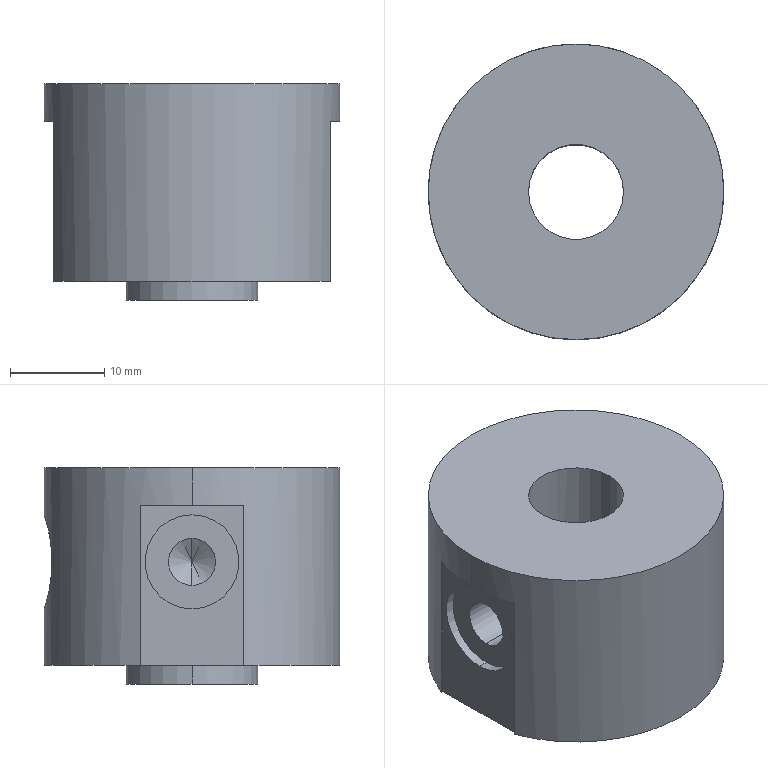Part | STEP file | 0229_Z_Cylinder_CG1DN25-75_2 | 1 solid | 54 faces | box 31.4 x 31.4 x 23 mm | volume 12832 mm3 | cylinder 26 | cone 14 | plane 14 | commonest cylinder face diameters 4.2 x8 10 x6 5 x4 6.8 x2 10.1 x2 14 x2